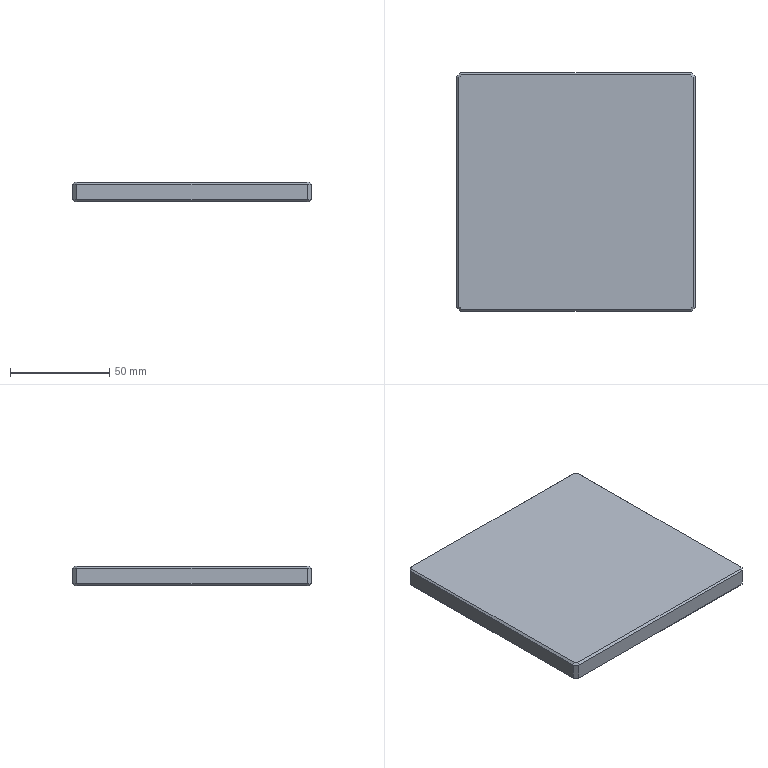Part | NX | 1 solid | 26 faces | box 120 x 120 x 10 mm | volume 143447 mm3 | plane 26
STEP:
#1=CARTESIAN_POINT('',(60.,-58.,9.));
#2=VERTEX_POINT('',#1);
#3=CARTESIAN_POINT('',(60.,-58.,1.));
#4=VERTEX_POINT('',#3);
#5=CARTESIAN_POINT('',(60.,-58.,10.));
#6=DIRECTION('',(0.,0.,-1.));
#7=VECTOR('',#6,1000.);
#8=LINE('',#5,#7);
#9=EDGE_CURVE('',#2,#4,#8,.T.);
#10=ORIENTED_EDGE('',*,*,#9,.T.);
#11=CARTESIAN_POINT('',(60.,58.,1.));
#12=VERTEX_POINT('',#11);
#13=CARTESIAN_POINT('',(60.,58.,1.));
#14=DIRECTION('',(0.,1.,0.));
#15=VECTOR('',#14,1000.);
#16=LINE('',#13,#15);
#17=EDGE_CURVE('',#4,#12,#16,.T.);
#18=ORIENTED_EDGE('',*,*,#17,.T.);
#19=CARTESIAN_POINT('',(60.,58.,9.));
#20=VERTEX_POINT('',#19);
#21=CARTESIAN_POINT('',(60.,58.,10.));
#22=DIRECTION('',(0.,0.,1.));
#23=VECTOR('',#22,1000.);
#24=LINE('',#21,#23);
#25=EDGE_CURVE('',#12,#20,#24,.T.);
#26=ORIENTED_EDGE('',*,*,#25,.T.);
#27=CARTESIAN_POINT('',(60.,-60.,9.));
#28=DIRECTION('',(0.,-1.,0.));
#29=VECTOR('',#28,1000.);
#30=LINE('',#27,#29);
#31=EDGE_CURVE('',#20,#2,#30,.T.);
#32=ORIENTED_EDGE('',*,*,#31,.T.);
#33=EDGE_LOOP('',(#10,#18,#26,#32));
#34=FACE_BOUND('',#33,.T.);
#35=CARTESIAN_POINT('',(60.,-60.,10.));
#36=DIRECTION('',(-1.,0.,0.));
#37=DIRECTION('',(0.,0.,1.));
#38=AXIS2_PLACEMENT_3D('',#35,#36,#37);
#39=PLANE('',#38);
#40=ADVANCED_FACE('',(#34),#39,.F.);
#41=CARTESIAN_POINT('',(58.,60.,9.));
#42=VERTEX_POINT('',#41);
#43=CARTESIAN_POINT('',(58.,60.,1.));
#44=VERTEX_POINT('',#43);
#45=CARTESIAN_POINT('',(58.,60.,10.));
#46=DIRECTION('',(0.,0.,-1.));
#47=VECTOR('',#46,1000.);
#48=LINE('',#45,#47);
#49=EDGE_CURVE('',#42,#44,#48,.T.);
#50=ORIENTED_EDGE('',*,*,#49,.T.);
#51=CARTESIAN_POINT('',(-58.,60.,1.));
#52=VERTEX_POINT('',#51);
#53=CARTESIAN_POINT('',(-58.,60.,1.));
#54=DIRECTION('',(-1.,0.,0.));
#55=VECTOR('',#54,1000.);
#56=LINE('',#53,#55);
#57=EDGE_CURVE('',#44,#52,#56,.T.);
#58=ORIENTED_EDGE('',*,*,#57,.T.);
#59=CARTESIAN_POINT('',(-58.,60.,9.));
#60=VERTEX_POINT('',#59);
#61=CARTESIAN_POINT('',(-58.,60.,10.));
#62=DIRECTION('',(0.,0.,1.));
#63=VECTOR('',#62,1000.);
#64=LINE('',#61,#63);
#65=EDGE_CURVE('',#52,#60,#64,.T.);
#66=ORIENTED_EDGE('',*,*,#65,.T.);
#67=CARTESIAN_POINT('',(-60.,60.,9.));
#68=DIRECTION('',(1.,0.,0.));
#69=VECTOR('',#68,1000.);
#70=LINE('',#67,#69);
#71=EDGE_CURVE('',#60,#42,#70,.T.);
#72=ORIENTED_EDGE('',*,*,#71,.T.);
#73=EDGE_LOOP('',(#50,#58,#66,#72));
#74=FACE_BOUND('',#73,.T.);
#75=CARTESIAN_POINT('',(-60.,60.,10.));
#76=DIRECTION('',(0.,-1.,0.));
#77=DIRECTION('',(0.,0.,-1.));
#78=AXIS2_PLACEMENT_3D('',#75,#76,#77);
#79=PLANE('',#78);
#80=ADVANCED_FACE('',(#74),#79,.F.);
#81=CARTESIAN_POINT('',(-60.,58.,9.));
#82=VERTEX_POINT('',#81);
#83=CARTESIAN_POINT('',(-60.,58.,1.));
#84=VERTEX_POINT('',#83);
#85=CARTESIAN_POINT('',(-60.,58.,10.));
#86=DIRECTION('',(0.,0.,-1.));
#87=VECTOR('',#86,1000.);
#88=LINE('',#85,#87);
#89=EDGE_CURVE('',#82,#84,#88,.T.);
#90=ORIENTED_EDGE('',*,*,#89,.T.);
#91=CARTESIAN_POINT('',(-60.,-58.,1.));
#92=VERTEX_POINT('',#91);
#93=CARTESIAN_POINT('',(-60.,-58.,1.));
#94=DIRECTION('',(0.,-1.,0.));
#95=VECTOR('',#94,1000.);
#96=LINE('',#93,#95);
#97=EDGE_CURVE('',#84,#92,#96,.T.);
#98=ORIENTED_EDGE('',*,*,#97,.T.);
#99=CARTESIAN_POINT('',(-60.,-58.,9.));
#100=VERTEX_POINT('',#99);
#101=CARTESIAN_POINT('',(-60.,-58.,10.));
#102=DIRECTION('',(0.,0.,1.));
#103=VECTOR('',#102,1000.);
#104=LINE('',#101,#103);
#105=EDGE_CURVE('',#92,#100,#104,.T.);
#106=ORIENTED_EDGE('',*,*,#105,.T.);
#107=CARTESIAN_POINT('',(-60.,-60.,9.));
#108=DIRECTION('',(0.,1.,0.));
#109=VECTOR('',#108,1000.);
#110=LINE('',#107,#109);
#111=EDGE_CURVE('',#100,#82,#110,.T.);
#112=ORIENTED_EDGE('',*,*,#111,.T.);
#113=EDGE_LOOP('',(#90,#98,#106,#112));
#114=FACE_BOUND('',#113,.T.);
#115=CARTESIAN_POINT('',(-60.,-60.,10.));
#116=DIRECTION('',(1.,0.,0.));
#117=DIRECTION('',(0.,1.,0.));
#118=AXIS2_PLACEMENT_3D('',#115,#116,#117);
#119=PLANE('',#118);
#120=ADVANCED_FACE('',(#114),#119,.F.);
#121=CARTESIAN_POINT('',(-58.,-60.,9.));
#122=VERTEX_POINT('',#121);
#123=CARTESIAN_POINT('',(-58.,-60.,1.));
#124=VERTEX_POINT('',#123);
#125=CARTESIAN_POINT('',(-58.,-60.,10.));
#126=DIRECTION('',(0.,0.,-1.));
#127=VECTOR('',#126,1000.);
#128=LINE('',#125,#127);
#129=EDGE_CURVE('',#122,#124,#128,.T.);
#130=ORIENTED_EDGE('',*,*,#129,.T.);
#131=CARTESIAN_POINT('',(58.,-60.,1.));
#132=VERTEX_POINT('',#131);
#133=CARTESIAN_POINT('',(58.,-60.,1.));
#134=DIRECTION('',(1.,0.,0.));
#135=VECTOR('',#134,1000.);
#136=LINE('',#133,#135);
#137=EDGE_CURVE('',#124,#132,#136,.T.);
#138=ORIENTED_EDGE('',*,*,#137,.T.);
#139=CARTESIAN_POINT('',(58.,-60.,9.));
#140=VERTEX_POINT('',#139);
#141=CARTESIAN_POINT('',(58.,-60.,10.));
#142=DIRECTION('',(0.,0.,1.));
#143=VECTOR('',#142,1000.);
#144=LINE('',#141,#143);
#145=EDGE_CURVE('',#132,#140,#144,.T.);
#146=ORIENTED_EDGE('',*,*,#145,.T.);
#147=CARTESIAN_POINT('',(-60.,-60.,9.));
#148=DIRECTION('',(-1.,0.,0.));
#149=VECTOR('',#148,1000.);
#150=LINE('',#147,#149);
#151=EDGE_CURVE('',#140,#122,#150,.T.);
#152=ORIENTED_EDGE('',*,*,#151,.T.);
#153=EDGE_LOOP('',(#130,#138,#146,#152));
#154=FACE_BOUND('',#153,.T.);
#155=CARTESIAN_POINT('',(-60.,-60.,10.));
#156=DIRECTION('',(0.,1.,0.));
#157=DIRECTION('',(0.,0.,1.));
#158=AXIS2_PLACEMENT_3D('',#155,#156,#157);
#159=PLANE('',#158);
#160=ADVANCED_FACE('',(#154),#159,.F.);
#161=CARTESIAN_POINT('',(57.586,59.,10.));
#162=VERTEX_POINT('',#161);
#163=CARTESIAN_POINT('',(-57.586,59.,10.));
#164=VERTEX_POINT('',#163);
#165=CARTESIAN_POINT('',(0.,59.,10.));
#166=DIRECTION('',(-1.,0.,0.));
#167=VECTOR('',#166,1000.);
#168=LINE('',#165,#167);
#169=EDGE_CURVE('',#162,#164,#168,.T.);
#170=ORIENTED_EDGE('',*,*,#169,.T.);
#171=CARTESIAN_POINT('',(-59.,57.586,10.));
#172=VERTEX_POINT('',#171);
#173=CARTESIAN_POINT('',(-59.293,57.293,10.));
#174=DIRECTION('',(-0.7071,-0.7071,0.));
#175=VECTOR('',#174,1000.);
#176=LINE('',#173,#175);
#177=EDGE_CURVE('',#164,#172,#176,.T.);
#178=ORIENTED_EDGE('',*,*,#177,.T.);
#179=CARTESIAN_POINT('',(-59.,-57.586,10.));
#180=VERTEX_POINT('',#179);
#181=CARTESIAN_POINT('',(-59.,0.,10.));
#182=DIRECTION('',(0.,-1.,0.));
#183=VECTOR('',#182,1000.);
#184=LINE('',#181,#183);
#185=EDGE_CURVE('',#172,#180,#184,.T.);
#186=ORIENTED_EDGE('',*,*,#185,.T.);
#187=CARTESIAN_POINT('',(-57.586,-59.,10.));
#188=VERTEX_POINT('',#187);
#189=CARTESIAN_POINT('',(-57.293,-59.293,10.));
#190=DIRECTION('',(0.7071,-0.7071,0.));
#191=VECTOR('',#190,1000.);
#192=LINE('',#189,#191);
#193=EDGE_CURVE('',#180,#188,#192,.T.);
#194=ORIENTED_EDGE('',*,*,#193,.T.);
#195=CARTESIAN_POINT('',(57.586,-59.,10.));
#196=VERTEX_POINT('',#195);
#197=CARTESIAN_POINT('',(0.,-59.,10.));
#198=DIRECTION('',(1.,0.,0.));
#199=VECTOR('',#198,1000.);
#200=LINE('',#197,#199);
#201=EDGE_CURVE('',#188,#196,#200,.T.);
#202=ORIENTED_EDGE('',*,*,#201,.T.);
#203=CARTESIAN_POINT('',(59.,-57.586,10.));
#204=VERTEX_POINT('',#203);
#205=CARTESIAN_POINT('',(59.293,-57.293,10.));
#206=DIRECTION('',(0.7071,0.7071,0.));
#207=VECTOR('',#206,1000.);
#208=LINE('',#205,#207);
#209=EDGE_CURVE('',#196,#204,#208,.T.);
#210=ORIENTED_EDGE('',*,*,#209,.T.);
#211=CARTESIAN_POINT('',(59.,57.586,10.));
#212=VERTEX_POINT('',#211);
#213=CARTESIAN_POINT('',(59.,0.,10.));
#214=DIRECTION('',(0.,1.,0.));
#215=VECTOR('',#214,1000.);
#216=LINE('',#213,#215);
#217=EDGE_CURVE('',#204,#212,#216,.T.);
#218=ORIENTED_EDGE('',*,*,#217,.T.);
#219=CARTESIAN_POINT('',(57.293,59.293,10.));
#220=DIRECTION('',(-0.7071,0.7071,0.));
#221=VECTOR('',#220,1000.);
#222=LINE('',#219,#221);
#223=EDGE_CURVE('',#212,#162,#222,.T.);
#224=ORIENTED_EDGE('',*,*,#223,.T.);
#225=EDGE_LOOP('',(#170,#178,#186,#194,#202,#210,#218,#224));
#226=FACE_BOUND('',#225,.T.);
#227=CARTESIAN_POINT('',(0.,0.,10.));
#228=DIRECTION('',(0.,0.,-1.));
#229=DIRECTION('',(-1.,0.,0.));
#230=AXIS2_PLACEMENT_3D('',#227,#228,#229);
#231=PLANE('',#230);
#232=ADVANCED_FACE('',(#226),#231,.F.);
#233=CARTESIAN_POINT('',(59.,57.586,0.));
#234=VERTEX_POINT('',#233);
#235=CARTESIAN_POINT('',(59.,-57.586,0.));
#236=VERTEX_POINT('',#235);
#237=CARTESIAN_POINT('',(59.,-58.,0.));
#238=DIRECTION('',(0.,-1.,0.));
#239=VECTOR('',#238,1000.);
#240=LINE('',#237,#239);
#241=EDGE_CURVE('',#234,#236,#240,.T.);
#242=ORIENTED_EDGE('',*,*,#241,.T.);
#243=CARTESIAN_POINT('',(57.586,-59.,0.));
#244=VERTEX_POINT('',#243);
#245=CARTESIAN_POINT('',(58.293,-58.293,0.));
#246=DIRECTION('',(-0.7071,-0.7071,0.));
#247=VECTOR('',#246,1000.);
#248=LINE('',#245,#247);
#249=EDGE_CURVE('',#236,#244,#248,.T.);
#250=ORIENTED_EDGE('',*,*,#249,.T.);
#251=CARTESIAN_POINT('',(-57.586,-59.,0.));
#252=VERTEX_POINT('',#251);
#253=CARTESIAN_POINT('',(-58.,-59.,0.));
#254=DIRECTION('',(-1.,0.,0.));
#255=VECTOR('',#254,1000.);
#256=LINE('',#253,#255);
#257=EDGE_CURVE('',#244,#252,#256,.T.);
#258=ORIENTED_EDGE('',*,*,#257,.T.);
#259=CARTESIAN_POINT('',(-59.,-57.586,0.));
#260=VERTEX_POINT('',#259);
#261=CARTESIAN_POINT('',(-58.293,-58.293,0.));
#262=DIRECTION('',(-0.7071,0.7071,0.));
#263=VECTOR('',#262,1000.);
#264=LINE('',#261,#263);
#265=EDGE_CURVE('',#252,#260,#264,.T.);
#266=ORIENTED_EDGE('',*,*,#265,.T.);
#267=CARTESIAN_POINT('',(-59.,57.586,0.));
#268=VERTEX_POINT('',#267);
#269=CARTESIAN_POINT('',(-59.,58.,0.));
#270=DIRECTION('',(0.,1.,0.));
#271=VECTOR('',#270,1000.);
#272=LINE('',#269,#271);
#273=EDGE_CURVE('',#260,#268,#272,.T.);
#274=ORIENTED_EDGE('',*,*,#273,.T.);
#275=CARTESIAN_POINT('',(-57.586,59.,0.));
#276=VERTEX_POINT('',#275);
#277=CARTESIAN_POINT('',(-58.293,58.293,0.));
#278=DIRECTION('',(0.7071,0.7071,0.));
#279=VECTOR('',#278,1000.);
#280=LINE('',#277,#279);
#281=EDGE_CURVE('',#268,#276,#280,.T.);
#282=ORIENTED_EDGE('',*,*,#281,.T.);
#283=CARTESIAN_POINT('',(57.586,59.,0.));
#284=VERTEX_POINT('',#283);
#285=CARTESIAN_POINT('',(58.,59.,0.));
#286=DIRECTION('',(1.,0.,0.));
#287=VECTOR('',#286,1000.);
#288=LINE('',#285,#287);
#289=EDGE_CURVE('',#276,#284,#288,.T.);
#290=ORIENTED_EDGE('',*,*,#289,.T.);
#291=CARTESIAN_POINT('',(58.293,58.293,0.));
#292=DIRECTION('',(0.7071,-0.7071,0.));
#293=VECTOR('',#292,1000.);
#294=LINE('',#291,#293);
#295=EDGE_CURVE('',#284,#234,#294,.T.);
#296=ORIENTED_EDGE('',*,*,#295,.T.);
#297=EDGE_LOOP('',(#242,#250,#258,#266,#274,#282,#290,#296));
#298=FACE_BOUND('',#297,.T.);
#299=CARTESIAN_POINT('',(0.,0.,0.));
#300=DIRECTION('',(0.,0.,-1.));
#301=DIRECTION('',(-1.,0.,0.));
#302=AXIS2_PLACEMENT_3D('',#299,#300,#301);
#303=PLANE('',#302);
#304=ADVANCED_FACE('',(#298),#303,.T.);
#305=ORIENTED_EDGE('',*,*,#105,.F.);
#306=CARTESIAN_POINT('',(-58.,-60.,1.));
#307=DIRECTION('',(-0.7071,0.7071,0.));
#308=VECTOR('',#307,1000.);
#309=LINE('',#306,#308);
#310=EDGE_CURVE('',#92,#124,#309,.F.);
#311=ORIENTED_EDGE('',*,*,#310,.T.);
#312=ORIENTED_EDGE('',*,*,#129,.F.);
#313=CARTESIAN_POINT('',(-60.,-58.,9.));
#314=DIRECTION('',(0.7071,-0.7071,0.));
#315=VECTOR('',#314,1000.);
#316=LINE('',#313,#315);
#317=EDGE_CURVE('',#122,#100,#316,.F.);
#318=ORIENTED_EDGE('',*,*,#317,.T.);
#319=EDGE_LOOP('',(#305,#311,#312,#318));
#320=FACE_BOUND('',#319,.T.);
#321=CARTESIAN_POINT('',(-58.,-60.,10.));
#322=DIRECTION('',(0.7071,0.7071,0.));
#323=DIRECTION('',(0.,0.,-1.));
#324=AXIS2_PLACEMENT_3D('',#321,#322,#323);
#325=PLANE('',#324);
#326=ADVANCED_FACE('',(#320),#325,.F.);
#327=ORIENTED_EDGE('',*,*,#145,.F.);
#328=CARTESIAN_POINT('',(60.,-58.,1.));
#329=DIRECTION('',(-0.7071,-0.7071,0.));
#330=VECTOR('',#329,1000.);
#331=LINE('',#328,#330);
#332=EDGE_CURVE('',#132,#4,#331,.F.);
#333=ORIENTED_EDGE('',*,*,#332,.T.);
#334=ORIENTED_EDGE('',*,*,#9,.F.);
#335=CARTESIAN_POINT('',(58.,-60.,9.));
#336=DIRECTION('',(0.7071,0.7071,0.));
#337=VECTOR('',#336,1000.);
#338=LINE('',#335,#337);
#339=EDGE_CURVE('',#2,#140,#338,.F.);
#340=ORIENTED_EDGE('',*,*,#339,.T.);
#341=EDGE_LOOP('',(#327,#333,#334,#340));
#342=FACE_BOUND('',#341,.T.);
#343=CARTESIAN_POINT('',(60.,-58.,10.));
#344=DIRECTION('',(-0.7071,0.7071,0.));
#345=DIRECTION('',(0.,0.,-1.));
#346=AXIS2_PLACEMENT_3D('',#343,#344,#345);
#347=PLANE('',#346);
#348=ADVANCED_FACE('',(#342),#347,.F.);
#349=ORIENTED_EDGE('',*,*,#25,.F.);
#350=CARTESIAN_POINT('',(58.,60.,1.));
#351=DIRECTION('',(0.7071,-0.7071,0.));
#352=VECTOR('',#351,1000.);
#353=LINE('',#350,#352);
#354=EDGE_CURVE('',#12,#44,#353,.F.);
#355=ORIENTED_EDGE('',*,*,#354,.T.);
#356=ORIENTED_EDGE('',*,*,#49,.F.);
#357=CARTESIAN_POINT('',(60.,58.,9.));
#358=DIRECTION('',(-0.7071,0.7071,0.));
#359=VECTOR('',#358,1000.);
#360=LINE('',#357,#359);
#361=EDGE_CURVE('',#42,#20,#360,.F.);
#362=ORIENTED_EDGE('',*,*,#361,.T.);
#363=EDGE_LOOP('',(#349,#355,#356,#362));
#364=FACE_BOUND('',#363,.T.);
#365=CARTESIAN_POINT('',(58.,60.,10.));
#366=DIRECTION('',(-0.7071,-0.7071,0.));
#367=DIRECTION('',(0.,0.,-1.));
#368=AXIS2_PLACEMENT_3D('',#365,#366,#367);
#369=PLANE('',#368);
#370=ADVANCED_FACE('',(#364),#369,.F.);
#371=ORIENTED_EDGE('',*,*,#65,.F.);
#372=CARTESIAN_POINT('',(-60.,58.,1.));
#373=DIRECTION('',(0.7071,0.7071,0.));
#374=VECTOR('',#373,1000.);
#375=LINE('',#372,#374);
#376=EDGE_CURVE('',#52,#84,#375,.F.);
#377=ORIENTED_EDGE('',*,*,#376,.T.);
#378=ORIENTED_EDGE('',*,*,#89,.F.);
#379=CARTESIAN_POINT('',(-58.,60.,9.));
#380=DIRECTION('',(-0.7071,-0.7071,0.));
#381=VECTOR('',#380,1000.);
#382=LINE('',#379,#381);
#383=EDGE_CURVE('',#82,#60,#382,.F.);
#384=ORIENTED_EDGE('',*,*,#383,.T.);
#385=EDGE_LOOP('',(#371,#377,#378,#384));
#386=FACE_BOUND('',#385,.T.);
#387=CARTESIAN_POINT('',(-60.,58.,10.));
#388=DIRECTION('',(0.7071,-0.7071,0.));
#389=DIRECTION('',(0.,0.,-1.));
#390=AXIS2_PLACEMENT_3D('',#387,#388,#389);
#391=PLANE('',#390);
#392=ADVANCED_FACE('',(#386),#391,.F.);
#393=CARTESIAN_POINT('',(-37.492,48.677,-21.508));
#394=DIRECTION('',(0.6786,-0.2811,-0.6786));
#395=VECTOR('',#394,1000.);
#396=LINE('',#393,#395);
#397=EDGE_CURVE('',#84,#268,#396,.T.);
#398=ORIENTED_EDGE('',*,*,#397,.F.);
#399=ORIENTED_EDGE('',*,*,#376,.F.);
#400=CARTESIAN_POINT('',(-57.507,58.809,-0.1907));
#401=DIRECTION('',(0.2811,-0.6786,-0.6786));
#402=VECTOR('',#401,1000.);
#403=LINE('',#400,#402);
#404=EDGE_CURVE('',#276,#52,#403,.F.);
#405=ORIENTED_EDGE('',*,*,#404,.F.);
#406=ORIENTED_EDGE('',*,*,#281,.F.);
#407=EDGE_LOOP('',(#398,#399,#405,#406));
#408=FACE_BOUND('',#407,.T.);
#409=CARTESIAN_POINT('',(-58.293,58.293,0.));
#410=DIRECTION('',(-0.5,0.5,-0.7071));
#411=DIRECTION('',(-0.7071,-0.7071,0.));
#412=AXIS2_PLACEMENT_3D('',#409,#410,#411);
#413=PLANE('',#412);
#414=ADVANCED_FACE('',(#408),#413,.T.);
#415=ORIENTED_EDGE('',*,*,#404,.T.);
#416=ORIENTED_EDGE('',*,*,#57,.F.);
#417=CARTESIAN_POINT('',(48.677,37.492,-21.508));
#418=DIRECTION('',(-0.2811,-0.6786,-0.6786));
#419=VECTOR('',#418,1000.);
#420=LINE('',#417,#419);
#421=EDGE_CURVE('',#284,#44,#420,.F.);
#422=ORIENTED_EDGE('',*,*,#421,.F.);
#423=ORIENTED_EDGE('',*,*,#289,.F.);
#424=EDGE_LOOP('',(#415,#416,#422,#423));
#425=FACE_BOUND('',#424,.T.);
#426=CARTESIAN_POINT('',(-60.,60.,1.));
#427=DIRECTION('',(0.,0.7071,-0.7071));
#428=DIRECTION('',(1.,0.,0.));
#429=AXIS2_PLACEMENT_3D('',#426,#427,#428);
#430=PLANE('',#429);
#431=ADVANCED_FACE('',(#425),#430,.T.);
#432=ORIENTED_EDGE('',*,*,#397,.T.);
#433=ORIENTED_EDGE('',*,*,#273,.F.);
#434=CARTESIAN_POINT('',(-58.809,-57.507,-0.1907));
#435=DIRECTION('',(0.6786,0.2811,-0.6786));
#436=VECTOR('',#435,1000.);
#437=LINE('',#434,#436);
#438=EDGE_CURVE('',#92,#260,#437,.T.);
#439=ORIENTED_EDGE('',*,*,#438,.F.);
#440=ORIENTED_EDGE('',*,*,#97,.F.);
#441=EDGE_LOOP('',(#432,#433,#439,#440));
#442=FACE_BOUND('',#441,.T.);
#443=CARTESIAN_POINT('',(-60.,-60.,1.));
#444=DIRECTION('',(-0.7071,0.,-0.7071));
#445=DIRECTION('',(0.,1.,0.));
#446=AXIS2_PLACEMENT_3D('',#443,#444,#445);
#447=PLANE('',#446);
#448=ADVANCED_FACE('',(#442),#447,.T.);
#449=ORIENTED_EDGE('',*,*,#421,.T.);
#450=ORIENTED_EDGE('',*,*,#354,.F.);
#451=CARTESIAN_POINT('',(58.809,57.507,-0.1907));
#452=DIRECTION('',(-0.6786,-0.2811,-0.6786));
#453=VECTOR('',#452,1000.);
#454=LINE('',#451,#453);
#455=EDGE_CURVE('',#234,#12,#454,.F.);
#456=ORIENTED_EDGE('',*,*,#455,.F.);
#457=ORIENTED_EDGE('',*,*,#295,.F.);
#458=EDGE_LOOP('',(#449,#450,#456,#457));
#459=FACE_BOUND('',#458,.T.);
#460=CARTESIAN_POINT('',(58.293,58.293,0.));
#461=DIRECTION('',(0.5,0.5,-0.7071));
#462=DIRECTION('',(-0.7071,0.7071,0.));
#463=AXIS2_PLACEMENT_3D('',#460,#461,#462);
#464=PLANE('',#463);
#465=ADVANCED_FACE('',(#459),#464,.T.);
#466=ORIENTED_EDGE('',*,*,#438,.T.);
#467=ORIENTED_EDGE('',*,*,#265,.F.);
#468=CARTESIAN_POINT('',(-58.158,-60.381,1.381));
#469=DIRECTION('',(0.2811,0.6786,-0.6786));
#470=VECTOR('',#469,1000.);
#471=LINE('',#468,#470);
#472=EDGE_CURVE('',#124,#252,#471,.T.);
#473=ORIENTED_EDGE('',*,*,#472,.F.);
#474=ORIENTED_EDGE('',*,*,#310,.F.);
#475=EDGE_LOOP('',(#466,#467,#473,#474));
#476=FACE_BOUND('',#475,.T.);
#477=CARTESIAN_POINT('',(-58.293,-58.293,0.));
#478=DIRECTION('',(-0.5,-0.5,-0.7071));
#479=DIRECTION('',(0.7071,-0.7071,0.));
#480=AXIS2_PLACEMENT_3D('',#477,#478,#479);
#481=PLANE('',#480);
#482=ADVANCED_FACE('',(#476),#481,.T.);
#483=ORIENTED_EDGE('',*,*,#455,.T.);
#484=ORIENTED_EDGE('',*,*,#17,.F.);
#485=CARTESIAN_POINT('',(60.381,-58.158,1.381));
#486=DIRECTION('',(-0.6786,0.2811,-0.6786));
#487=VECTOR('',#486,1000.);
#488=LINE('',#485,#487);
#489=EDGE_CURVE('',#236,#4,#488,.F.);
#490=ORIENTED_EDGE('',*,*,#489,.F.);
#491=ORIENTED_EDGE('',*,*,#241,.F.);
#492=EDGE_LOOP('',(#483,#484,#490,#491));
#493=FACE_BOUND('',#492,.T.);
#494=CARTESIAN_POINT('',(60.,-60.,1.));
#495=DIRECTION('',(0.7071,0.,-0.7071));
#496=DIRECTION('',(0.,-1.,0.));
#497=AXIS2_PLACEMENT_3D('',#494,#495,#496);
#498=PLANE('',#497);
#499=ADVANCED_FACE('',(#493),#498,.T.);
#500=ORIENTED_EDGE('',*,*,#472,.T.);
#501=ORIENTED_EDGE('',*,*,#257,.F.);
#502=CARTESIAN_POINT('',(48.677,-37.492,-21.508));
#503=DIRECTION('',(0.2811,-0.6786,0.6786));
#504=VECTOR('',#503,1000.);
#505=LINE('',#502,#504);
#506=EDGE_CURVE('',#132,#244,#505,.F.);
#507=ORIENTED_EDGE('',*,*,#506,.F.);
#508=ORIENTED_EDGE('',*,*,#137,.F.);
#509=EDGE_LOOP('',(#500,#501,#507,#508));
#510=FACE_BOUND('',#509,.T.);
#511=CARTESIAN_POINT('',(-60.,-60.,1.));
#512=DIRECTION('',(0.,-0.7071,-0.7071));
#513=DIRECTION('',(-1.,0.,0.));
#514=AXIS2_PLACEMENT_3D('',#511,#512,#513);
#515=PLANE('',#514);
#516=ADVANCED_FACE('',(#510),#515,.T.);
#517=ORIENTED_EDGE('',*,*,#489,.T.);
#518=ORIENTED_EDGE('',*,*,#332,.F.);
#519=ORIENTED_EDGE('',*,*,#506,.T.);
#520=ORIENTED_EDGE('',*,*,#249,.F.);
#521=EDGE_LOOP('',(#517,#518,#519,#520));
#522=FACE_BOUND('',#521,.T.);
#523=CARTESIAN_POINT('',(58.293,-58.293,0.));
#524=DIRECTION('',(0.5,-0.5,-0.7071));
#525=DIRECTION('',(0.7071,0.7071,0.));
#526=AXIS2_PLACEMENT_3D('',#523,#524,#525);
#527=PLANE('',#526);
#528=ADVANCED_FACE('',(#522),#527,.T.);
#529=CARTESIAN_POINT('',(53.036,-48.016,20.984));
#530=DIRECTION('',(-0.2811,0.6786,0.6786));
#531=VECTOR('',#530,1000.);
#532=LINE('',#529,#531);
#533=EDGE_CURVE('',#140,#196,#532,.T.);
#534=ORIENTED_EDGE('',*,*,#533,.F.);
#535=ORIENTED_EDGE('',*,*,#339,.F.);
#536=CARTESIAN_POINT('',(58.809,-57.507,10.191));
#537=DIRECTION('',(-0.6786,0.2811,0.6786));
#538=VECTOR('',#537,1000.);
#539=LINE('',#536,#538);
#540=EDGE_CURVE('',#204,#2,#539,.F.);
#541=ORIENTED_EDGE('',*,*,#540,.F.);
#542=ORIENTED_EDGE('',*,*,#209,.F.);
#543=EDGE_LOOP('',(#534,#535,#541,#542));
#544=FACE_BOUND('',#543,.T.);
#545=CARTESIAN_POINT('',(58.293,-58.293,10.));
#546=DIRECTION('',(-0.5,0.5,-0.7071));
#547=DIRECTION('',(0.7071,0.7071,0.));
#548=AXIS2_PLACEMENT_3D('',#545,#546,#547);
#549=PLANE('',#548);
#550=ADVANCED_FACE('',(#544),#549,.F.);
#551=ORIENTED_EDGE('',*,*,#540,.T.);
#552=ORIENTED_EDGE('',*,*,#31,.F.);
#553=CARTESIAN_POINT('',(48.016,53.036,20.984));
#554=DIRECTION('',(-0.6786,-0.2811,0.6786));
#555=VECTOR('',#554,1000.);
#556=LINE('',#553,#555);
#557=EDGE_CURVE('',#212,#20,#556,.F.);
#558=ORIENTED_EDGE('',*,*,#557,.F.);
#559=ORIENTED_EDGE('',*,*,#217,.F.);
#560=EDGE_LOOP('',(#551,#552,#558,#559));
#561=FACE_BOUND('',#560,.T.);
#562=CARTESIAN_POINT('',(59.,0.,10.));
#563=DIRECTION('',(-0.7071,0.,-0.7071));
#564=DIRECTION('',(0.,1.,0.));
#565=AXIS2_PLACEMENT_3D('',#562,#563,#564);
#566=PLANE('',#565);
#567=ADVANCED_FACE('',(#561),#566,.F.);
#568=ORIENTED_EDGE('',*,*,#533,.T.);
#569=ORIENTED_EDGE('',*,*,#201,.F.);
#570=CARTESIAN_POINT('',(-57.507,-58.809,10.191));
#571=DIRECTION('',(0.2811,0.6786,0.6786));
#572=VECTOR('',#571,1000.);
#573=LINE('',#570,#572);
#574=EDGE_CURVE('',#122,#188,#573,.T.);
#575=ORIENTED_EDGE('',*,*,#574,.F.);
#576=ORIENTED_EDGE('',*,*,#151,.F.);
#577=EDGE_LOOP('',(#568,#569,#575,#576));
#578=FACE_BOUND('',#577,.T.);
#579=CARTESIAN_POINT('',(0.,-59.,10.));
#580=DIRECTION('',(0.,0.7071,-0.7071));
#581=DIRECTION('',(1.,0.,0.));
#582=AXIS2_PLACEMENT_3D('',#579,#580,#581);
#583=PLANE('',#582);
#584=ADVANCED_FACE('',(#578),#583,.F.);
#585=ORIENTED_EDGE('',*,*,#557,.T.);
#586=ORIENTED_EDGE('',*,*,#361,.F.);
#587=CARTESIAN_POINT('',(57.507,58.809,10.191));
#588=DIRECTION('',(-0.2811,-0.6786,0.6786));
#589=VECTOR('',#588,1000.);
#590=LINE('',#587,#589);
#591=EDGE_CURVE('',#162,#42,#590,.F.);
#592=ORIENTED_EDGE('',*,*,#591,.F.);
#593=ORIENTED_EDGE('',*,*,#223,.F.);
#594=EDGE_LOOP('',(#585,#586,#592,#593));
#595=FACE_BOUND('',#594,.T.);
#596=CARTESIAN_POINT('',(58.293,58.293,10.));
#597=DIRECTION('',(-0.5,-0.5,-0.7071));
#598=DIRECTION('',(-0.7071,0.7071,0.));
#599=AXIS2_PLACEMENT_3D('',#596,#597,#598);
#600=PLANE('',#599);
#601=ADVANCED_FACE('',(#595),#600,.F.);
#602=ORIENTED_EDGE('',*,*,#574,.T.);
#603=ORIENTED_EDGE('',*,*,#193,.F.);
#604=CARTESIAN_POINT('',(-48.016,-53.036,20.984));
#605=DIRECTION('',(0.6786,0.2811,0.6786));
#606=VECTOR('',#605,1000.);
#607=LINE('',#604,#606);
#608=EDGE_CURVE('',#100,#180,#607,.T.);
#609=ORIENTED_EDGE('',*,*,#608,.F.);
#610=ORIENTED_EDGE('',*,*,#317,.F.);
#611=EDGE_LOOP('',(#602,#603,#609,#610));
#612=FACE_BOUND('',#611,.T.);
#613=CARTESIAN_POINT('',(-58.293,-58.293,10.));
#614=DIRECTION('',(0.5,0.5,-0.7071));
#615=DIRECTION('',(0.7071,-0.7071,0.));
#616=AXIS2_PLACEMENT_3D('',#613,#614,#615);
#617=PLANE('',#616);
#618=ADVANCED_FACE('',(#612),#617,.F.);
#619=ORIENTED_EDGE('',*,*,#591,.T.);
#620=ORIENTED_EDGE('',*,*,#71,.F.);
#621=CARTESIAN_POINT('',(-53.036,48.016,20.984));
#622=DIRECTION('',(0.2811,-0.6786,0.6786));
#623=VECTOR('',#622,1000.);
#624=LINE('',#621,#623);
#625=EDGE_CURVE('',#164,#60,#624,.F.);
#626=ORIENTED_EDGE('',*,*,#625,.F.);
#627=ORIENTED_EDGE('',*,*,#169,.F.);
#628=EDGE_LOOP('',(#619,#620,#626,#627));
#629=FACE_BOUND('',#628,.T.);
#630=CARTESIAN_POINT('',(0.,59.,10.));
#631=DIRECTION('',(0.,-0.7071,-0.7071));
#632=DIRECTION('',(-1.,0.,0.));
#633=AXIS2_PLACEMENT_3D('',#630,#631,#632);
#634=PLANE('',#633);
#635=ADVANCED_FACE('',(#629),#634,.F.);
#636=ORIENTED_EDGE('',*,*,#608,.T.);
#637=ORIENTED_EDGE('',*,*,#185,.F.);
#638=CARTESIAN_POINT('',(-48.016,53.036,20.984));
#639=DIRECTION('',(-0.6786,0.2811,-0.6786));
#640=VECTOR('',#639,1000.);
#641=LINE('',#638,#640);
#642=EDGE_CURVE('',#82,#172,#641,.F.);
#643=ORIENTED_EDGE('',*,*,#642,.F.);
#644=ORIENTED_EDGE('',*,*,#111,.F.);
#645=EDGE_LOOP('',(#636,#637,#643,#644));
#646=FACE_BOUND('',#645,.T.);
#647=CARTESIAN_POINT('',(-59.,0.,10.));
#648=DIRECTION('',(0.7071,0.,-0.7071));
#649=DIRECTION('',(0.,-1.,0.));
#650=AXIS2_PLACEMENT_3D('',#647,#648,#649);
#651=PLANE('',#650);
#652=ADVANCED_FACE('',(#646),#651,.F.);
#653=ORIENTED_EDGE('',*,*,#625,.T.);
#654=ORIENTED_EDGE('',*,*,#383,.F.);
#655=ORIENTED_EDGE('',*,*,#642,.T.);
#656=ORIENTED_EDGE('',*,*,#177,.F.);
#657=EDGE_LOOP('',(#653,#654,#655,#656));
#658=FACE_BOUND('',#657,.T.);
#659=CARTESIAN_POINT('',(-58.293,58.293,10.));
#660=DIRECTION('',(0.5,-0.5,-0.7071));
#661=DIRECTION('',(-0.7071,-0.7071,0.));
#662=AXIS2_PLACEMENT_3D('',#659,#660,#661);
#663=PLANE('',#662);
#664=ADVANCED_FACE('',(#658),#663,.F.);
#665=CLOSED_SHELL('',(#40,#80,#120,#160,#232,#304,#326,#348,#370,#392,#414,#431,#448,#465,#482,#499,#516,#528,#550,#567,#584,#601,#618,#635,#652,#664));
#666=MANIFOLD_SOLID_BREP('',#665);
#667=(LENGTH_UNIT()NAMED_UNIT(*)SI_UNIT(.MILLI.,.METRE.));
#668=UNCERTAINTY_MEASURE_WITH_UNIT(LENGTH_MEASURE(0.00001),#667,'','');
#669=(NAMED_UNIT(*)PLANE_ANGLE_UNIT()SI_UNIT($,.RADIAN.));
#670=(NAMED_UNIT(*)SI_UNIT($,.STERADIAN.)SOLID_ANGLE_UNIT());
#671=(GEOMETRIC_REPRESENTATION_CONTEXT(3)GLOBAL_UNCERTAINTY_ASSIGNED_CONTEXT((#668))GLOBAL_UNIT_ASSIGNED_CONTEXT((#667,#669,#670))REPRESENTATION_CONTEXT('',''));
#672=ADVANCED_BREP_SHAPE_REPRESENTATION('',(#666),#671);